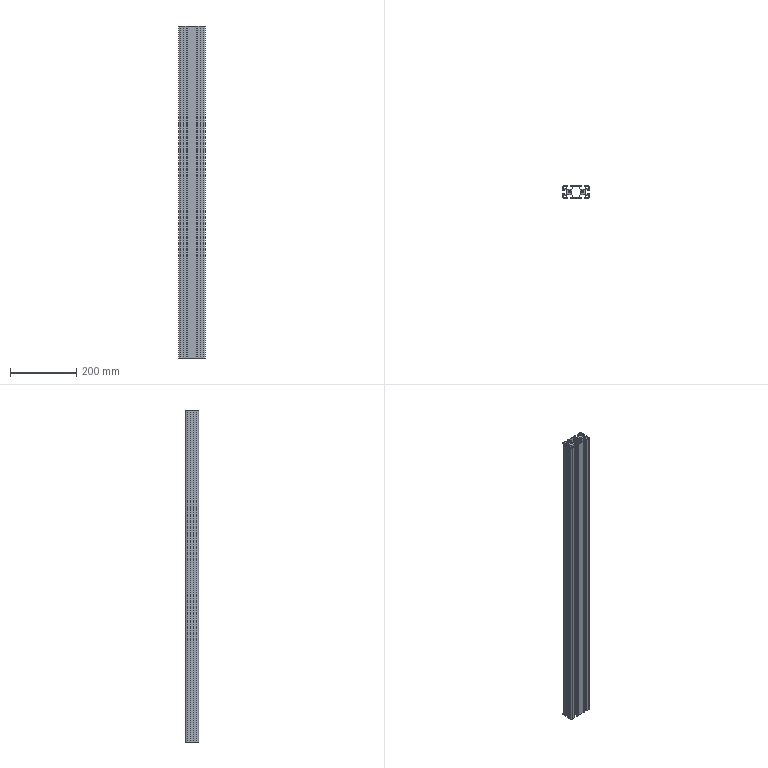Part | SolidWorks | features Fillet 2, Extrusion 1 | 1 solid | 170 faces | box 80 x 40 x 1000 mm | volume 1063867 mm3 | plane 142 | cylinder 28 | commonest cylinder face diameters 2 x16 10 x8 6.5 x4